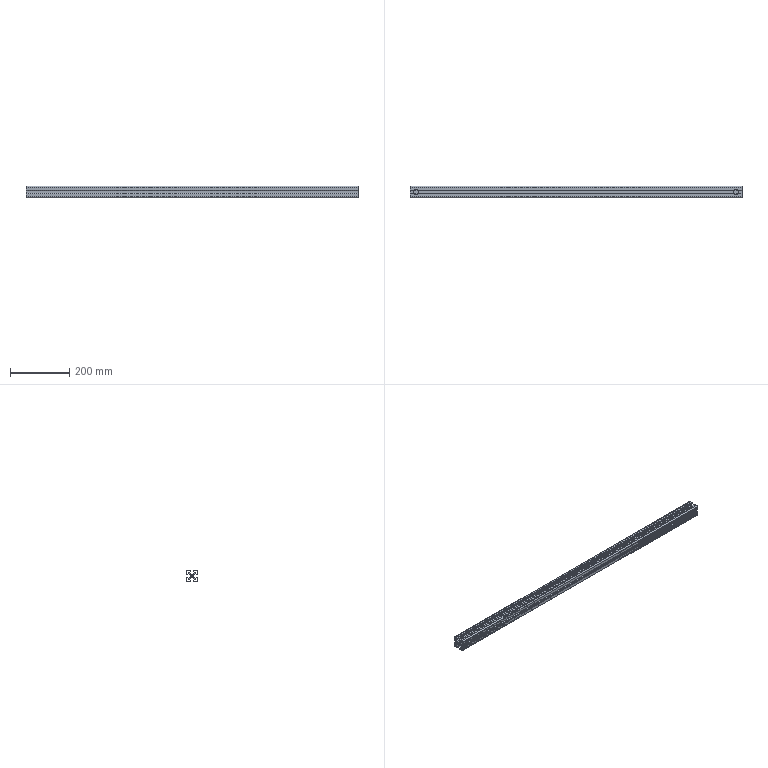Part | STEP file | 1 solid | 316 faces | box 1120 x 40 x 40 mm | volume 531368 mm3 | cylinder 166 | plane 150 | commonest cylinder face diameters 0.6 x62 2 x36 4 x24 0.4 x16 19 x16 6 x4